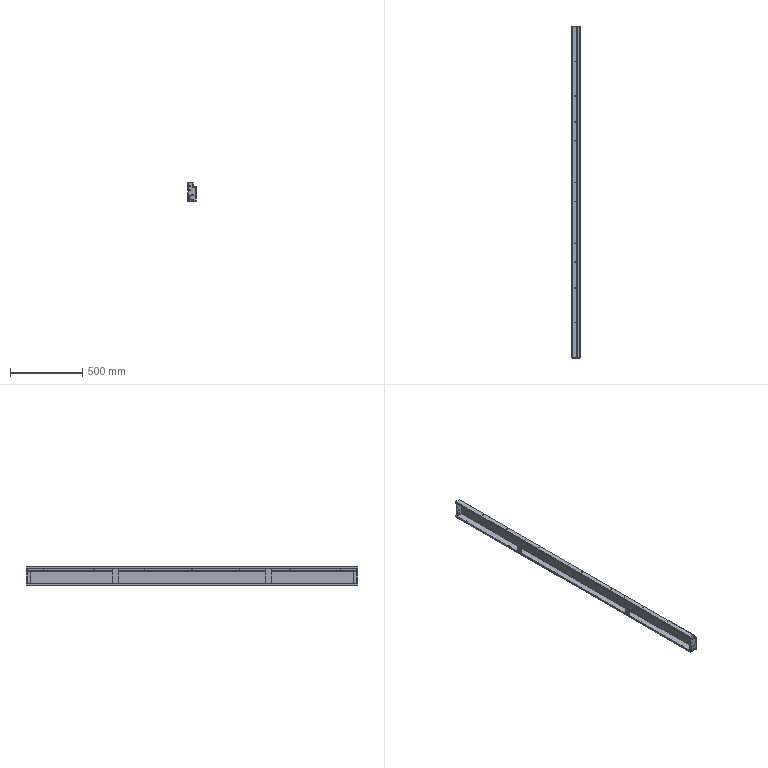Part | 5 solids | 222 faces | box 58 x 2300 x 130 mm | volume 766806 mm3 | plane 122 | cylinder 100 | commonest cylinder face diameters 5 x32 8 x20 9 x18 4.6 x14 2 x10 4.4 x6